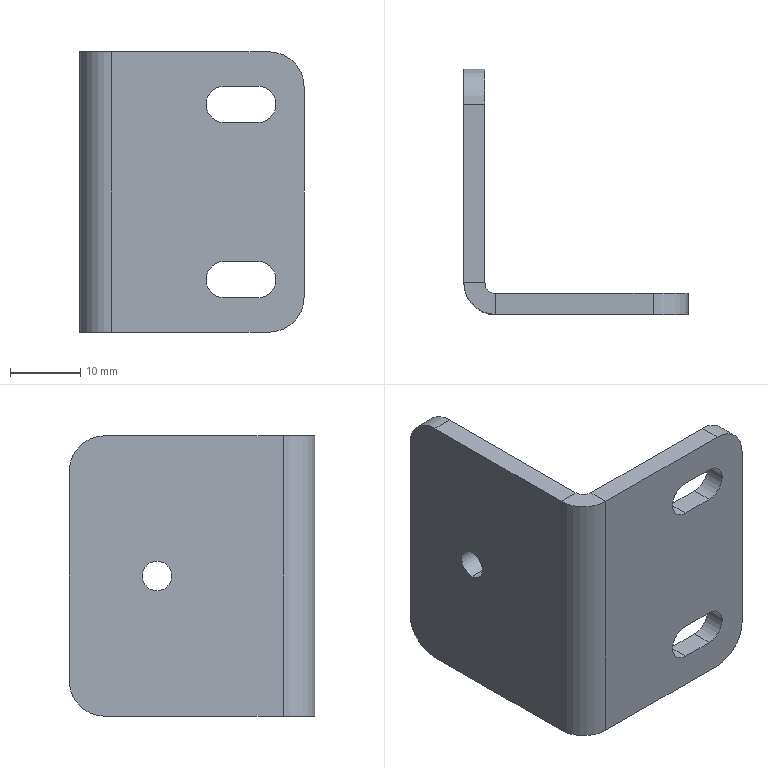Part | STEP file | Adapter plate 3 | 1 solid | 28 faces | box 32 x 35 x 40 mm | volume 7142 mm3 | plane 16 | cylinder 12 | commonest cylinder face diameters 5.2 x4 10 x4 4.2 x2 3 x1 9 x1